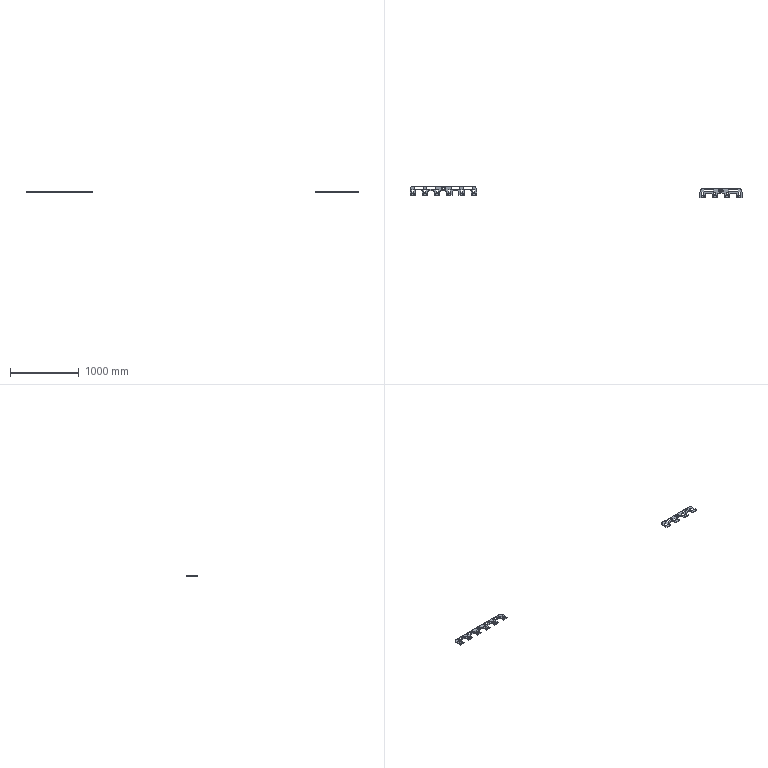NC program | NX | posted with a generic post | part box 4825 x 168.213 x 13 mm
Lines 13349 to 14244 of 14244:
(PLANAR_MILL_COPY_1 , TOOL : D6A45)
N26636 T07 M6
N26638 G54
N26640 G17 G0 G90 X915. Y-2.73 S9500 M3
N26642 G43 Z30. H7
N26644 Z0.
N26646 G94 G1 Z-1. F1400.
N26648 X914.3 Y-3.134
N26650 G3 X913.8 Y-4. R1.
N26652 G1 Y-21.
N26654 G3 X915.9 Y-23.1 R2.1
N26656 G1 X939.9
N26658 G3 X942. Y-21. R2.1
N26660 G1 Y13.
N26662 G3 X939.9 Y15.1 R2.1
N26664 G1 X915.9
N26666 G3 X913.8 Y13. R2.1
N26668 G1 Y-4.
N26670 G3 X914.3 Y-4.866 R1.
N26672 G1 X915. Y-5.27
N26674 Z0.
N26676 G0 Z30.
N26678 X840.27 Y54.9
N26680 Z0.
N26682 G1 Z-1.
N26684 X839.866 Y55.6
N26686 G3 X839. Y56.1 R1.
N26688 G1 X778.1
N26690 G3 X776. Y54. R2.1
N26692 G1 Y28.
N26694 G3 X778.1 Y25.9 R2.1
N26696 G1 X899.9
N26698 G3 X902. Y28. R2.1
N26700 G1 Y54.
N26702 G3 X899.9 Y56.1 R2.1
N26704 G1 X839.
N26706 G3 X838.134 Y55.6 R1.
N26708 G1 X837.73 Y54.9
N26710 Z0.
N26712 G0 Z30.
N26714 X763. Y-5.27
N26716 Z0.
N26718 G1 Z-1.
N26720 X763.7 Y-4.866
N26722 G3 X764.2 Y-4. R1.
N26724 G1 Y13.
N26726 G3 X762.1 Y15.1 R2.1
N26728 G1 X738.1
N26730 G3 X736. Y13. R2.1
N26732 G1 Y-21.
N26734 G3 X738.1 Y-23.1 R2.1
N26736 G1 X762.1
N26738 G3 X764.2 Y-21. R2.1
N26740 G1 Y-4.
N26742 G3 X763.7 Y-3.134 R1.
N26744 G1 X763. Y-2.73
N26746 Z0.
N26748 G0 Z30.
N26750 X662.47 Y54.9
N26752 Z0.
N26754 G1 Z-1.
N26756 X662.066 Y55.6
N26758 G3 X661.2 Y56.1 R1.
N26760 G1 X600.3
N26762 G3 X598.2 Y54. R2.1
N26764 G1 Y28.
N26766 G3 X600.3 Y25.9 R2.1
N26768 G1 X722.1
N26770 G3 X724.2 Y28. R2.1
N26772 G1 Y54.
N26774 G3 X722.1 Y56.1 R2.1
N26776 G1 X661.2
N26778 G3 X660.334 Y55.6 R1.
N26780 G1 X659.93 Y54.9
N26782 Z0.
N26784 G0 Z30.
N26786 X585.2 Y-5.27
N26788 Z0.
N26790 G1 Z-1.
N26792 X585.9 Y-4.866
N26794 G3 X586.4 Y-4. R1.
N26796 G1 Y13.
N26798 G3 X584.3 Y15.1 R2.1
N26800 G1 X560.3
N26802 G3 X558.2 Y13. R2.1
N26804 G1 Y-21.
N26806 G3 X560.3 Y-23.1 R2.1
N26808 G1 X584.3
N26810 G3 X586.4 Y-21. R2.1
N26812 G1 Y-4.
N26814 G3 X585.9 Y-3.134 R1.
N26816 G1 X585.2 Y-2.73
N26818 Z0.
N26820 G0 Z30.
N26822 X482.13 Y69.1
N26824 Z0.
N26826 G1 Z-1.
N26828 X482.534 Y68.4
N26830 G3 X483.4 Y67.9 R1.
N26832 G1 X916.8
N26834 G2 X967.7 Y17. R50.9
N26836 G1 Y-33.3
N26838 G2 X966.7 Y-34.3 R1.
N26840 G1 X889.1
N26842 G2 X888.1 Y-33.3 R1.
N26844 G1 Y-5.
N26846 G3 X869. Y14.1 R19.1
N26848 G1 X809.
N26850 G3 X789.9 Y-5. R19.1
N26852 G1 Y-33.3
N26854 G2 X788.9 Y-34.3 R1.
N26856 G1 X711.3
N26858 G2 X710.3 Y-33.3 R1.
N26860 G1 Y-20.95
N26862 G3 X691.2 Y-1.85 R19.1
N26864 G1 X631.2
N26866 G3 X612.1 Y-20.95 R19.1
N26868 G1 Y-33.3
N26870 G2 X611.1 Y-34.3 R1.
N26872 G1 X533.5
N26874 G2 X532.5 Y-33.3 R1.
N26876 G1 Y-20.95
N26878 G3 X513.4 Y-1.85 R19.1
N26880 G1 X453.4
N26882 G3 X434.3 Y-20.95 R19.1
N26884 G1 Y-33.3
N26886 G2 X433.3 Y-34.3 R1.
N26888 G1 X355.7
N26890 G2 X354.7 Y-33.3 R1.
N26892 G1 Y-20.95
N26894 G3 X335.6 Y-1.85 R19.1
N26896 G1 X275.6
N26898 G3 X256.5 Y-20.95 R19.1
N26900 G1 Y-33.3
N26902 G2 X255.5 Y-34.3 R1.
N26904 G1 X177.9
N26906 G2 X176.9 Y-33.3 R1.
N26908 G1 Y-5.
N26910 G3 X157.8 Y14.1 R19.1
N26912 G1 X97.8
N26914 G3 X78.7 Y-5. R19.1
N26916 G1 Y-33.3
N26918 G2 X77.7 Y-34.3 R1.
N26920 G1 X0.1
N26922 G2 X-0.9 Y-33.3 R1.
N26924 G1 Y17.
N26926 G2 X50. Y67.9 R50.9
N26928 G1 X483.4
N26930 G3 X484.266 Y68.4 R1.
N26932 G1 X484.67 Y69.1
N26934 Z0.
N26936 G0 Z30.
N26938 X493.515 Y5.329
N26940 Z0.
N26942 G1 Z-1.
N26944 X493.249 Y4.531
N26946 G3 X494.115 Y4.031 R1.
N26948 X497.215 Y7.131 R3.1
N26950 X494.115 Y4.031 R-3.1
N26952 X494.981 Y4.531 R1.
N26954 G1 X494.716 Y5.329
N26956 Z0.
N26958 G0 Z30.
N26960 X472.084
N26962 Z0.
N26964 G1 Z-1.
N26966 X471.819 Y4.531
N26968 G3 X472.685 Y4.031 R1.
N26970 X475.785 Y7.131 R3.1
N26972 X472.685 Y4.031 R-3.1
N26974 X473.551 Y4.531 R1.
N26976 G1 X473.285 Y5.329
N26978 Z0.
N26980 G0 Z30.
N26982 X484.709 Y45.833
N26984 Z0.
N26986 G1 Z-1.
N26988 X484.266 Y46.6
N26990 G3 X483.4 Y47.1 R1.
N26992 X469.3 Y33. R14.1
N26994 X483.4 Y47.1 R-14.1
N26996 X482.534 Y46.6 R1.
N26998 G1 X482.091 Y45.833
N27000 Z0.
N27002 G0 Z30.
N27004 X509.869 Y24.087
N27006 Z0.
N27008 G1 Z-1.
N27010 X510.135 Y24.885
N27012 G3 X509.269 Y25.385 R1.
N27014 X506.169 Y22.285 R3.1
N27016 X509.269 Y25.385 R-3.1
N27018 X508.403 Y24.885 R1.
N27020 G1 X508.668 Y24.087
N27022 Z0.
N27024 G0 Z30.
N27026 X509.869 Y45.518
N27028 Z0.
N27030 G1 Z-1.
N27032 X510.135 Y46.315
N27034 G3 X509.269 Y46.815 R1.
N27036 X506.169 Y43.715 R3.1
N27038 X509.269 Y46.815 R-3.1
N27040 X508.403 Y46.315 R1.
N27042 G1 X508.668 Y45.518
N27044 Z0.
N27046 G0 Z30.
N27048 X494.716 Y60.671
N27050 Z0.
N27052 G1 Z-1.
N27054 X494.981 Y61.469
N27056 G3 X494.115 Y61.969 R1.
N27058 X491.015 Y58.869 R3.1
N27060 X494.115 Y61.969 R-3.1
N27062 X493.249 Y61.469 R1.
N27064 G1 X493.515 Y60.671
N27066 Z0.
N27068 G0 Z30.
N27070 X473.285
N27072 Z0.
N27074 G1 Z-1.
N27076 X473.551 Y61.469
N27078 G3 X472.685 Y61.969 R1.
N27080 X469.585 Y58.869 R3.1
N27082 X472.685 Y61.969 R-3.1
N27084 X471.819 Y61.469 R1.
N27086 G1 X472.084 Y60.671
N27088 Z0.
N27090 G0 Z30.
N27092 X458.132 Y45.518
N27094 Z0.
N27096 G1 Z-1.
N27098 X458.397 Y46.315
N27100 G3 X457.531 Y46.815 R1.
N27102 X454.431 Y43.715 R3.1
N27104 X457.531 Y46.815 R-3.1
N27106 X456.665 Y46.315 R1.
N27108 G1 X456.931 Y45.518
N27110 Z0.
N27112 G0 Z30.
N27114 X458.132 Y24.087
N27116 Z0.
N27118 G1 Z-1.
N27120 X458.397 Y24.885
N27122 G3 X457.531 Y25.385 R1.
N27124 X454.431 Y22.285 R3.1
N27126 X457.531 Y25.385 R-3.1
N27128 X456.665 Y24.885 R1.
N27130 G1 X456.931 Y24.087
N27132 Z0.
N27134 G0 Z30.
N27136 X407.4 Y-5.27
N27138 Z0.
N27140 G1 Z-1.
N27142 X408.1 Y-4.866
N27144 G3 X408.6 Y-4. R1.
N27146 G1 Y13.
N27148 G3 X406.5 Y15.1 R2.1
N27150 G1 X382.5
N27152 G3 X380.4 Y13. R2.1
N27154 G1 Y-21.
N27156 G3 X382.5 Y-23.1 R2.1
N27158 G1 X406.5
N27160 G3 X408.6 Y-21. R2.1
N27162 G1 Y-4.
N27164 G3 X408.1 Y-3.134 R1.
N27166 G1 X407.4 Y-2.73
N27168 Z0.
N27170 G0 Z30.
N27172 X306.87 Y54.9
N27174 Z0.
N27176 G1 Z-1.
N27178 X306.466 Y55.6
N27180 G3 X305.6 Y56.1 R1.
N27182 G1 X244.7
N27184 G3 X242.6 Y54. R2.1
N27186 G1 Y28.
N27188 G3 X244.7 Y25.9 R2.1
N27190 G1 X366.5
N27192 G3 X368.6 Y28. R2.1
N27194 G1 Y54.
N27196 G3 X366.5 Y56.1 R2.1
N27198 G1 X305.6
N27200 G3 X304.734 Y55.6 R1.
N27202 G1 X304.33 Y54.9
N27204 Z0.
N27206 G0 Z30.
N27208 X229.6 Y-5.27
N27210 Z0.
N27212 G1 Z-1.
N27214 X230.3 Y-4.866
N27216 G3 X230.8 Y-4. R1.
N27218 G1 Y13.
N27220 G3 X228.7 Y15.1 R2.1
N27222 G1 X204.7
N27224 G3 X202.6 Y13. R2.1
N27226 G1 Y-21.
N27228 G3 X204.7 Y-23.1 R2.1
N27230 G1 X228.7
N27232 G3 X230.8 Y-21. R2.1
N27234 G1 Y-4.
N27236 G3 X230.3 Y-3.134 R1.
N27238 G1 X229.6 Y-2.73
N27240 Z0.
N27242 G0 Z30.
N27244 X129.07 Y54.9
N27246 Z0.
N27248 G1 Z-1.
N27250 X128.666 Y55.6
N27252 G3 X127.8 Y56.1 R1.
N27254 G1 X66.9
N27256 G3 X64.8 Y54. R2.1
N27258 G1 Y28.
N27260 G3 X66.9 Y25.9 R2.1
N27262 G1 X188.7
N27264 G3 X190.8 Y28. R2.1
N27266 G1 Y54.
N27268 G3 X188.7 Y56.1 R2.1
N27270 G1 X127.8
N27272 G3 X126.934 Y55.6 R1.
N27274 G1 X126.53 Y54.9
N27276 Z0.
N27278 G0 Z30.
N27280 X51.8 Y-5.27
N27282 Z0.
N27284 G1 Z-1.
N27286 X52.5 Y-4.866
N27288 G3 X53. Y-4. R1.
N27290 G1 Y13.
N27292 G3 X50.9 Y15.1 R2.1
N27294 G1 X26.9
N27296 G3 X24.8 Y13. R2.1
N27298 G1 Y-21.
N27300 G3 X26.9 Y-23.1 R2.1
N27302 G1 X50.9
N27304 G3 X53. Y-21. R2.1
N27306 G1 Y-4.
N27308 G3 X52.5 Y-3.134 R1.
N27310 G1 X51.8 Y-2.73
N27312 Z0.
N27314 G0 Z30.
(PLANAR_MILL_COPY_COPY , TOOL : D6A45)
N27316 X18.412 Y-62.242
N27318 Z-3.
N27320 G1 Z-4.
N27322 X18.034 Y-63.05
N27324 G3 X18.9 Y-63.55 R1.
N27326 X21.25 Y-61.2 R2.35
N27328 X18.9 Y-63.55 R-2.35
N27330 X19.766 Y-63.05 R1.
N27332 G1 X19.388 Y-62.242
N27334 Z-3.
N27336 G0 Z30.
N27338 X18.893 Y-38.1
N27340 Z-3.
N27342 G1 Z-4.
N27344 Y-37.056
N27346 G3 X18.418 Y-36.9 R0.5
N27348 X19.382 Y-36.9 R-2.35
N27350 X18.907 Y-37.056 R0.5
N27352 G1 Y-38.1
N27354 Z-3.
N27356 G0 Z30.
N27358 X58.893
N27360 Z-3.
N27362 G1 Z-4.
N27364 Y-37.056
N27366 G3 X58.418 Y-36.9 R0.5
N27368 X59.382 Y-36.9 R-2.35
N27370 X58.907 Y-37.056 R0.5
N27372 G1 Y-38.1
N27374 Z-3.
N27376 G0 Z30.
N27378 X58.412 Y-62.242
N27380 Z-3.
N27382 G1 Z-4.
N27384 X58.034 Y-63.05
N27386 G3 X58.9 Y-63.55 R1.
N27388 X61.25 Y-61.2 R2.35
N27390 X58.9 Y-63.55 R-2.35
N27392 X59.766 Y-63.05 R1.
N27394 G1 X59.388 Y-62.242
N27396 Z-3.
N27398 G0 Z30.
N27400 X196.212
N27402 Z-3.
N27404 G1 Z-4.
N27406 X195.834 Y-63.05
N27408 G3 X196.7 Y-63.55 R1.
N27410 X199.05 Y-61.2 R2.35
N27412 X196.7 Y-63.55 R-2.35
N27414 X197.566 Y-63.05 R1.
N27416 G1 X197.188 Y-62.242
N27418 Z-3.
N27420 G0 Z30.
N27422 X196.693 Y-38.1
N27424 Z-3.
N27426 G1 Z-4.
N27428 Y-37.056
N27430 G3 X196.218 Y-36.9 R0.5
N27432 X197.182 Y-36.9 R-2.35
N27434 X196.707 Y-37.056 R0.5
N27436 G1 Y-38.1
N27438 Z-3.
N27440 G0 Z30.
N27442 X236.693
N27444 Z-3.
N27446 G1 Z-4.
N27448 Y-37.056
N27450 G3 X236.218 Y-36.9 R0.5
N27452 X237.182 Y-36.9 R-2.35
N27454 X236.707 Y-37.056 R0.5
N27456 G1 Y-38.1
N27458 Z-3.
N27460 G0 Z30.
N27462 X236.212 Y-62.242
N27464 Z-3.
N27466 G1 Z-4.
N27468 X235.834 Y-63.05
N27470 G3 X236.7 Y-63.55 R1.
N27472 X239.05 Y-61.2 R2.35
N27474 X236.7 Y-63.55 R-2.35
N27476 X237.566 Y-63.05 R1.
N27478 G1 X237.188 Y-62.242
N27480 Z-3.
N27482 G0 Z30.
N27484 X374.012
N27486 Z-3.
N27488 G1 Z-4.
N27490 X373.634 Y-63.05
N27492 G3 X374.5 Y-63.55 R1.
N27494 X376.85 Y-61.2 R2.35
N27496 X374.5 Y-63.55 R-2.35
N27498 X375.366 Y-63.05 R1.
N27500 G1 X374.988 Y-62.242
N27502 Z-3.
N27504 G0 Z30.
N27506 X374.493 Y-38.1
N27508 Z-3.
N27510 G1 Z-4.
N27512 Y-37.056
N27514 G3 X374.018 Y-36.9 R0.5
N27516 X374.982 Y-36.9 R-2.35
N27518 X374.507 Y-37.056 R0.5
N27520 G1 Y-38.1
N27522 Z-3.
N27524 G0 Z30.
N27526 X414.493
N27528 Z-3.
N27530 G1 Z-4.
N27532 Y-37.056
N27534 G3 X414.018 Y-36.9 R0.5
N27536 X414.982 Y-36.9 R-2.35
N27538 X414.507 Y-37.056 R0.5
N27540 G1 Y-38.1
N27542 Z-3.
N27544 G0 Z30.
N27546 X414.012 Y-62.242
N27548 Z-3.
N27550 G1 Z-4.
N27552 X413.634 Y-63.05
N27554 G3 X414.5 Y-63.55 R1.
N27556 X416.85 Y-61.2 R2.35
N27558 X414.5 Y-63.55 R-2.35
N27560 X415.366 Y-63.05 R1.
N27562 G1 X414.988 Y-62.242
N27564 Z-3.
N27566 G0 Z30.
N27568 X435.713 Y-37.492
N27570 Z-3.
N27572 G1 Z-4.
N27574 X435.265 Y-37.043
N27576 G3 X434.3 Y-36.782 R1.
N27578 G1 Y-66.9
N27580 G2 X433.3 Y-67.9 R1.
N27582 G1 X355.7
N27584 G2 X354.7 Y-66.9 R1.
N27586 G1 Y-36.782
N27588 G3 X353.735 Y-37.043 R1.
N27590 G1 X353.287 Y-37.492
N27592 Z-3.
N27594 G0 Z30.
N27596 X257.913
N27598 Z-3.
N27600 G1 Z-4.
N27602 X257.465 Y-37.043
N27604 G3 X256.5 Y-36.782 R1.
N27606 G1 Y-66.9
N27608 G2 X255.5 Y-67.9 R1.
N27610 G1 X177.9
N27612 G2 X176.9 Y-66.9 R1.
N27614 G1 Y-36.782
N27616 G3 X175.935 Y-37.043 R1.
N27618 G1 X175.487 Y-37.492
N27620 Z-3.
N27622 G0 Z30.
N27624 X80.113
N27626 Z-3.
N27628 G1 Z-4.
N27630 X79.665 Y-37.043
N27632 G3 X78.7 Y-36.782 R1.
N27634 G1 Y-66.9
N27636 G2 X77.7 Y-67.9 R1.
N27638 G1 X0.1
N27640 G2 X-0.9 Y-66.9 R1.
N27642 G1 Y-36.782
N27644 G3 X-1.865 Y-37.043 R1.
N27646 G1 X-2.313 Y-37.492
N27648 Z-3.
N27650 G0 Z30.
N27652 X969.113
N27654 Z-3.
N27656 G1 Z-4.
N27658 X968.665 Y-37.043
N27660 G3 X967.7 Y-36.782 R1.
N27662 G1 Y-66.9
N27664 G2 X966.7 Y-67.9 R1.
N27666 G1 X889.1
N27668 G2 X888.1 Y-66.9 R1.
N27670 G1 Y-36.782
N27672 G3 X887.135 Y-37.043 R1.
N27674 G1 X886.687 Y-37.492
N27676 Z-3.
N27678 G0 Z30.
N27680 X791.313
N27682 Z-3.
N27684 G1 Z-4.
N27686 X790.865 Y-37.043
N27688 G3 X789.9 Y-36.782 R1.
N27690 G1 Y-66.9
N27692 G2 X788.9 Y-67.9 R1.
N27694 G1 X711.3
N27696 G2 X710.3 Y-66.9 R1.
N27698 G1 Y-36.782
N27700 G3 X709.335 Y-37.043 R1.
N27702 G1 X708.887 Y-37.492
N27704 Z-3.
N27706 G0 Z30.
N27708 X613.513
N27710 Z-3.
N27712 G1 Z-4.
N27714 X613.065 Y-37.043
N27716 G3 X612.1 Y-36.782 R1.
N27718 G1 Y-66.9
N27720 G2 X611.1 Y-67.9 R1.
N27722 G1 X533.5
N27724 G2 X532.5 Y-66.9 R1.
N27726 G1 Y-36.782
N27728 G3 X531.535 Y-37.043 R1.
N27730 G1 X531.087 Y-37.492
N27732 Z-3.
N27734 G0 Z30.
N27736 X551.812 Y-62.242
N27738 Z-3.
N27740 G1 Z-4.
N27742 X551.434 Y-63.05
N27744 G3 X552.3 Y-63.55 R1.
N27746 X554.65 Y-61.2 R2.35
N27748 X552.3 Y-63.55 R-2.35
N27750 X553.166 Y-63.05 R1.
N27752 G1 X552.788 Y-62.242
N27754 Z-3.
N27756 G0 Z30.
N27758 X552.293 Y-38.1
N27760 Z-3.
N27762 G1 Z-4.
N27764 Y-37.056
N27766 G3 X551.818 Y-36.9 R0.5
N27768 X552.782 Y-36.9 R-2.35
N27770 X552.307 Y-37.056 R0.5
N27772 G1 Y-38.1
N27774 Z-3.
N27776 G0 Z30.
N27778 X592.293
N27780 Z-3.
N27782 G1 Z-4.
N27784 Y-37.056
N27786 G3 X591.818 Y-36.9 R0.5
N27788 X592.782 Y-36.9 R-2.35
N27790 X592.307 Y-37.056 R0.5
N27792 G1 Y-38.1
N27794 Z-3.
N27796 G0 Z30.
N27798 X591.812 Y-62.242
N27800 Z-3.
N27802 G1 Z-4.
N27804 X591.434 Y-63.05
N27806 G3 X592.3 Y-63.55 R1.
N27808 X594.65 Y-61.2 R2.35
N27810 X592.3 Y-63.55 R-2.35
N27812 X593.166 Y-63.05 R1.
N27814 G1 X592.788 Y-62.242
N27816 Z-3.
N27818 G0 Z30.
N27820 X729.612
N27822 Z-3.
N27824 G1 Z-4.
N27826 X729.234 Y-63.05
N27828 G3 X730.1 Y-63.55 R1.
N27830 X732.45 Y-61.2 R2.35
N27832 X730.1 Y-63.55 R-2.35
N27834 X730.966 Y-63.05 R1.
N27836 G1 X730.588 Y-62.242
N27838 Z-3.
N27840 G0 Z30.
N27842 X730.093 Y-38.1
N27844 Z-3.
N27846 G1 Z-4.
N27848 Y-37.056
N27850 G3 X729.618 Y-36.9 R0.5
N27852 X730.582 Y-36.9 R-2.35
N27854 X730.107 Y-37.056 R0.5
N27856 G1 Y-38.1
N27858 Z-3.
N27860 G0 Z30.
N27862 X770.093
N27864 Z-3.
N27866 G1 Z-4.
N27868 Y-37.056
N27870 G3 X769.618 Y-36.9 R0.5
N27872 X770.582 Y-36.9 R-2.35
N27874 X770.107 Y-37.056 R0.5
N27876 G1 Y-38.1
N27878 Z-3.
N27880 G0 Z30.
N27882 X769.612 Y-62.242
N27884 Z-3.
N27886 G1 Z-4.
N27888 X769.234 Y-63.05
N27890 G3 X770.1 Y-63.55 R1.
N27892 X772.45 Y-61.2 R2.35
N27894 X770.1 Y-63.55 R-2.35
N27896 X770.966 Y-63.05 R1.
N27898 G1 X770.588 Y-62.242
N27900 Z-3.
N27902 G0 Z30.
N27904 X907.412
N27906 Z-3.
N27908 G1 Z-4.
N27910 X907.034 Y-63.05
N27912 G3 X907.9 Y-63.55 R1.
N27914 X910.25 Y-61.2 R2.35
N27916 X907.9 Y-63.55 R-2.35
N27918 X908.766 Y-63.05 R1.
N27920 G1 X908.388 Y-62.242
N27922 Z-3.
N27924 G0 Z30.
N27926 X907.893 Y-38.1
N27928 Z-3.
N27930 G1 Z-4.
N27932 Y-37.056
N27934 G3 X907.418 Y-36.9 R0.5
N27936 X908.382 Y-36.9 R-2.35
N27938 X907.907 Y-37.056 R0.5
N27940 G1 Y-38.1
N27942 Z-3.
N27944 G0 Z30.
N27946 X947.893
N27948 Z-3.
N27950 G1 Z-4.
N27952 Y-37.056
N27954 G3 X947.418 Y-36.9 R0.5
N27956 X948.382 Y-36.9 R-2.35
N27958 X947.907 Y-37.056 R0.5
N27960 G1 Y-38.1
N27962 Z-3.
N27964 G0 Z30.
N27966 X947.412 Y-62.242
N27968 Z-3.
N27970 G1 Z-4.
N27972 X947.034 Y-63.05
N27974 G3 X947.9 Y-63.55 R1.
N27976 X950.25 Y-61.2 R2.35
N27978 X947.9 Y-63.55 R-2.35
N27980 X948.766 Y-63.05 R1.
N27982 G1 X948.388 Y-62.242
N27984 Z-3.
N27986 G0 Z30.
N27988 M5
(ZLEVEL_PROFILE_COPY_3_COPY , TOOL : D10)
N27990 T10 M6
N27992 G54
N27994 G17 G0 G90 X47.434 Y75.444 S9500 M3
N27996 G43 Z30. H10
N27998 Z-7.525
N28000 G94 G1 Z-12.525 F1000.
N28002 X49.134 Y72.5
N28004 G3 X50. Y72. R1.
N28006 G1 X916.8 F1200.
N28008 G2 X971.8 Y17. R55.
N28010 G1 Y-67.
N28012 G2 X966.8 Y-72. R5.
N28014 G1 X889.
N28016 G2 X884. Y-67. R5.
N28018 G1 Y-5.
N28020 G3 X869. Y10. R15.
N28022 G1 X809.
N28024 G3 X794. Y-5. R15.
N28026 G1 Y-67.
N28028 G2 X789. Y-72. R5.
N28030 G1 X711.2
N28032 G2 X706.2 Y-67. R5.
N28034 G1 Y-20.95
N28036 G3 X691.2 Y-5.95 R15.
N28038 G1 X631.2
N28040 G3 X616.2 Y-20.95 R15.
N28042 G1 Y-67.
N28044 G2 X611.2 Y-72. R5.
N28046 G1 X533.4
N28048 G2 X528.4 Y-67. R5.
N28050 G1 Y-20.95
N28052 G3 X513.4 Y-5.95 R15.
N28054 G1 X453.4
N28056 G3 X438.4 Y-20.95 R15.
N28058 G1 Y-67.
N28060 G2 X433.4 Y-72. R5.
N28062 G1 X355.6
N28064 G2 X350.6 Y-67. R5.
N28066 G1 Y-20.95
N28068 G3 X335.6 Y-5.95 R15.
N28070 G1 X275.6
N28072 G3 X260.6 Y-20.95 R15.
N28074 G1 Y-67.
N28076 G2 X255.6 Y-72. R5.
N28078 G1 X177.8
N28080 G2 X172.8 Y-67. R5.
N28082 G1 Y-5.
N28084 G3 X157.8 Y10. R15.
N28086 G1 X97.8
N28088 G3 X82.8 Y-5. R15.
N28090 G1 Y-67.
N28092 G2 X77.8 Y-72. R5.
N28094 G1 X0.
N28096 G2 X-5. Y-67. R5.
N28098 G1 Y17.
N28100 G2 X50. Y72. R55.
N28102 G1 X57.161 Z-12.65
N28104 X916.8
N28106 G2 X971.8 Y17. R55.
N28108 G1 Y-67.
N28110 G2 X966.8 Y-72. R5.
N28112 G1 X889.
N28114 G2 X884. Y-67. R5.
N28116 G1 Y-5.
N28118 G3 X869. Y10. R15.
N28120 G1 X809.
N28122 G3 X794. Y-5. R15.
N28124 G1 Y-67.
N28126 G2 X789. Y-72. R5.
N28128 G1 X711.2
N28130 G2 X706.2 Y-67. R5.
N28132 G1 Y-20.95
N28134 G3 X691.2 Y-5.95 R15.
N28136 G1 X631.2
N28138 G3 X616.2 Y-20.95 R15.
N28140 G1 Y-67.
N28142 G2 X611.2 Y-72. R5.
N28144 G1 X533.4
N28146 G2 X528.4 Y-67. R5.
N28148 G1 Y-20.95
N28150 G3 X513.4 Y-5.95 R15.
N28152 G1 X453.4
N28154 G3 X438.4 Y-20.95 R15.
N28156 G1 Y-67.
N28158 G2 X433.4 Y-72. R5.
N28160 G1 X355.6
N28162 G2 X350.6 Y-67. R5.
N28164 G1 Y-20.95
N28166 G3 X335.6 Y-5.95 R15.
N28168 G1 X275.6
N28170 G3 X260.6 Y-20.95 R15.
N28172 G1 Y-67.
N28174 G2 X255.6 Y-72. R5.
N28176 G1 X177.8
N28178 G2 X172.8 Y-67. R5.
N28180 G1 Y-5.
N28182 G3 X157.8 Y10. R15.
N28184 G1 X97.8
N28186 G3 X82.8 Y-5. R15.
N28188 G1 Y-67.
N28190 G2 X77.8 Y-72. R5.
N28192 G1 X0.
N28194 G2 X-5. Y-67. R5.
N28196 G1 Y17.
N28198 G2 X50. Y72. R55.
N28200 G1 X57.161 Z-12.775
N28202 X916.8
N28204 G2 X971.8 Y17. R55.
N28206 G1 Y-67.
N28208 G2 X966.8 Y-72. R5.
N28210 G1 X889.
N28212 G2 X884. Y-67. R5.
N28214 G1 Y-5.
N28216 G3 X869. Y10. R15.
N28218 G1 X809.
N28220 G3 X794. Y-5. R15.
N28222 G1 Y-67.
N28224 G2 X789. Y-72. R5.
N28226 G1 X711.2
N28228 G2 X706.2 Y-67. R5.
N28230 G1 Y-20.95
N28232 G3 X691.2 Y-5.95 R15.
N28234 G1 X631.2
N28236 G3 X616.2 Y-20.95 R15.
N28238 G1 Y-67.
N28240 G2 X611.2 Y-72. R5.
N28242 G1 X533.4
N28244 G2 X528.4 Y-67. R5.
N28246 G1 Y-20.95
N28248 G3 X513.4 Y-5.95 R15.
N28250 G1 X453.4
N28252 G3 X438.4 Y-20.95 R15.
N28254 G1 Y-67.
N28256 G2 X433.4 Y-72. R5.
N28258 G1 X355.6
N28260 G2 X350.6 Y-67. R5.
N28262 G1 Y-20.95
N28264 G3 X335.6 Y-5.95 R15.
N28266 G1 X275.6
N28268 G3 X260.6 Y-20.95 R15.
N28270 G1 Y-67.
N28272 G2 X255.6 Y-72. R5.
N28274 G1 X177.8
N28276 G2 X172.8 Y-67. R5.
N28278 G1 Y-5.
N28280 G3 X157.8 Y10. R15.
N28282 G1 X97.8
N28284 G3 X82.8 Y-5. R15.
N28286 G1 Y-67.
N28288 G2 X77.8 Y-72. R5.
N28290 G1 X0.
N28292 G2 X-5. Y-67. R5.
N28294 G1 Y17.
N28296 G2 X50. Y72. R55.
N28298 G1 X57.161 Z-12.9
N28300 X916.8
N28302 G2 X971.8 Y17. R55.
N28304 G1 Y-67.
N28306 G2 X966.8 Y-72. R5.
N28308 G1 X889.
N28310 G2 X884. Y-67. R5.
N28312 G1 Y-5.
N28314 G3 X869. Y10. R15.
N28316 G1 X809.
N28318 G3 X794. Y-5. R15.
N28320 G1 Y-67.
N28322 G2 X789. Y-72. R5.
N28324 G1 X711.2
N28326 G2 X706.2 Y-67. R5.
N28328 G1 Y-20.95
N28330 G3 X691.2 Y-5.95 R15.
N28332 G1 X631.2
N28334 G3 X616.2 Y-20.95 R15.
N28336 G1 Y-67.
N28338 G2 X611.2 Y-72. R5.
N28340 G1 X533.4
N28342 G2 X528.4 Y-67. R5.
N28344 G1 Y-20.95
N28346 G3 X513.4 Y-5.95 R15.
N28348 G1 X453.4
N28350 G3 X438.4 Y-20.95 R15.
N28352 G1 Y-67.
N28354 G2 X433.4 Y-72. R5.
N28356 G1 X355.6
N28358 G2 X350.6 Y-67. R5.
N28360 G1 Y-20.95
N28362 G3 X335.6 Y-5.95 R15.
N28364 G1 X275.6
N28366 G3 X260.6 Y-20.95 R15.
N28368 G1 Y-67.
N28370 G2 X255.6 Y-72. R5.
N28372 G1 X177.8
N28374 G2 X172.8 Y-67. R5.
N28376 G1 Y-5.
N28378 G3 X157.8 Y10. R15.
N28380 G1 X97.8
N28382 G3 X82.8 Y-5. R15.
N28384 G1 Y-67.
N28386 G2 X77.8 Y-72. R5.
N28388 G1 X0.
N28390 G2 X-5. Y-67. R5.
N28392 G1 Y17.
N28394 G2 X50. Y72. R55.
N28396 G1 X57.161
N28398 G3 X58.027 Y72.5 R1.
N28400 G1 X59.759 Y75.5
N28402 Z-7.9
N28404 G0 Z30.
N28406 M5
N28408 M2